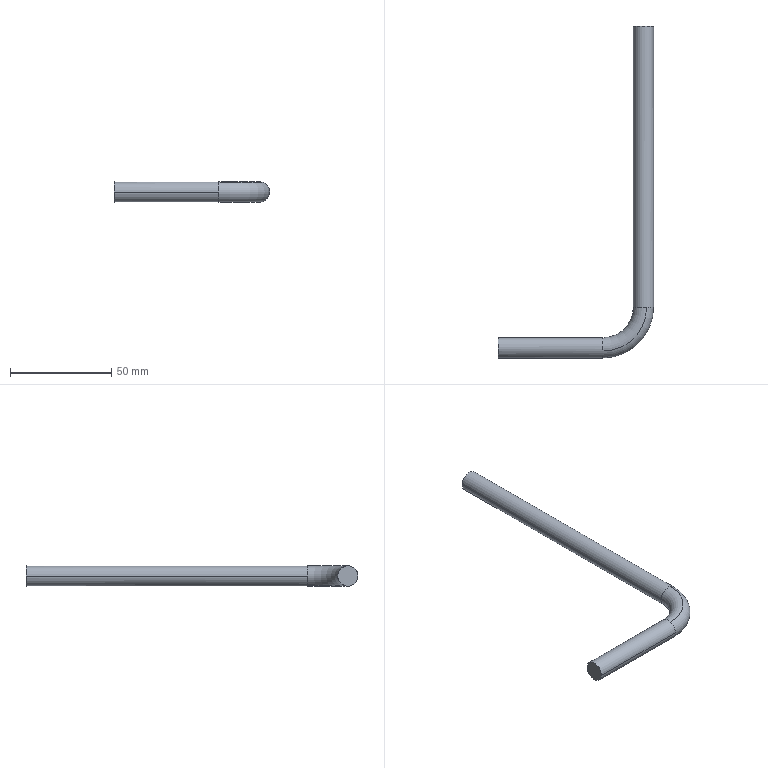Part | 1 solid | 8 faces | box 76.634 x 163.975 x 10 mm | volume 17438 mm3 | cylinder 4 | plane 2 | torus 2 | commonest cylinder face diameters 10 x4
STEP:
#1=CARTESIAN_POINT('',(0.,0.,0.));
#2=DIRECTION('',(0.,0.,1.));
#3=DIRECTION('',(1.,0.,0.));
#4=AXIS2_PLACEMENT_3D('',#1,#2,#3);
#5=CARTESIAN_POINT('',(-430.236,381.551,-68.051));
#6=VERTEX_POINT('',#5);
#7=CARTESIAN_POINT('',(-430.236,520.526,-68.051));
#8=VERTEX_POINT('',#7);
#9=CARTESIAN_POINT('',(-430.236,381.551,-68.051));
#10=DIRECTION('',(0.,1.,0.));
#11=VECTOR('',#10,1.);
#12=LINE('',#9,#11);
#13=CARTESIAN_POINT('',(-425.236,381.551,-68.051));
#14=DIRECTION('',(0.,1.,0.));
#15=DIRECTION('',(0.,0.,-1.));
#16=AXIS2_PLACEMENT_3D('',#13,#14,#15);
#17=CYLINDRICAL_SURFACE('',#16,5.);
#18=CARTESIAN_POINT('',(1.571,0.));
#19=DIRECTION('',(0.,1.));
#20=VECTOR('',#19,1.);
#21=LINE('',#18,#20);
#22=(GEOMETRIC_REPRESENTATION_CONTEXT(2)PARAMETRIC_REPRESENTATION_CONTEXT()REPRESENTATION_CONTEXT('',''));
#23=DEFINITIONAL_REPRESENTATION('',(#21),#22);
#24=PCURVE('',#17,#23);
#25=CARTESIAN_POINT('',(-425.236,381.551,-68.051));
#26=DIRECTION('',(0.,1.,0.));
#27=DIRECTION('',(0.,0.,1.));
#28=AXIS2_PLACEMENT_3D('',#25,#26,#27);
#29=CYLINDRICAL_SURFACE('',#28,5.);
#30=CARTESIAN_POINT('',(4.712,0.));
#31=DIRECTION('',(0.,1.));
#32=VECTOR('',#31,1.);
#33=LINE('',#30,#32);
#34=(GEOMETRIC_REPRESENTATION_CONTEXT(2)PARAMETRIC_REPRESENTATION_CONTEXT()REPRESENTATION_CONTEXT('',''));
#35=DEFINITIONAL_REPRESENTATION('',(#33),#34);
#36=PCURVE('',#29,#35);
#37=SURFACE_CURVE('',#12,(#24,#36),.PCURVE_S1.);
#38=EDGE_CURVE('',#6,#8,#37,.T.);
#39=ORIENTED_EDGE('',*,*,#38,.F.);
#40=CARTESIAN_POINT('',(-423.691,381.551,-63.296));
#41=VERTEX_POINT('',#40);
#42=CARTESIAN_POINT('',(-425.236,381.551,-68.051));
#43=DIRECTION('',(0.,1.,0.));
#44=DIRECTION('',(1.,0.,0.));
#45=AXIS2_PLACEMENT_3D('',#42,#43,#44);
#46=CIRCLE('',#45,5.);
#47=CARTESIAN_POINT('',(-1.571,0.));
#48=DIRECTION('',(1.,0.));
#49=VECTOR('',#48,1.);
#50=LINE('',#47,#49);
#51=(GEOMETRIC_REPRESENTATION_CONTEXT(2)PARAMETRIC_REPRESENTATION_CONTEXT()REPRESENTATION_CONTEXT('',''));
#52=DEFINITIONAL_REPRESENTATION('',(#50),#51);
#53=PCURVE('',#17,#52);
#54=CARTESIAN_POINT('',(-445.236,381.551,-68.051));
#55=DIRECTION('',(0.,0.,1.));
#56=DIRECTION('',(-0.7071,0.7071,0.));
#57=AXIS2_PLACEMENT_3D('',#54,#55,#56);
#58=TOROIDAL_SURFACE('',#57,20.,5.);
#59=CARTESIAN_POINT('',(3.927,6.283));
#60=DIRECTION('',(0.,-1.));
#61=VECTOR('',#60,1.);
#62=LINE('',#59,#61);
#63=(GEOMETRIC_REPRESENTATION_CONTEXT(2)PARAMETRIC_REPRESENTATION_CONTEXT()REPRESENTATION_CONTEXT('',''));
#64=DEFINITIONAL_REPRESENTATION('',(#62),#63);
#65=PCURVE('',#58,#64);
#66=SURFACE_CURVE('',#46,(#53,#65),.PCURVE_S1.);
#67=EDGE_CURVE('',#6,#41,#66,.T.);
#68=ORIENTED_EDGE('',*,*,#67,.T.);
#69=CARTESIAN_POINT('',(-420.236,381.551,-68.051));
#70=VERTEX_POINT('',#69);
#71=CARTESIAN_POINT('',(-425.236,381.551,-68.051));
#72=DIRECTION('',(0.,1.,0.));
#73=DIRECTION('',(1.,0.,0.));
#74=AXIS2_PLACEMENT_3D('',#71,#72,#73);
#75=CIRCLE('',#74,5.);
#76=CARTESIAN_POINT('',(-1.571,0.));
#77=DIRECTION('',(1.,0.));
#78=VECTOR('',#77,1.);
#79=LINE('',#76,#78);
#80=(GEOMETRIC_REPRESENTATION_CONTEXT(2)PARAMETRIC_REPRESENTATION_CONTEXT()REPRESENTATION_CONTEXT('',''));
#81=DEFINITIONAL_REPRESENTATION('',(#79),#80);
#82=PCURVE('',#17,#81);
#83=CARTESIAN_POINT('',(-445.236,381.551,-68.051));
#84=DIRECTION('',(0.,0.,1.));
#85=DIRECTION('',(-0.7071,0.7071,0.));
#86=AXIS2_PLACEMENT_3D('',#83,#84,#85);
#87=TOROIDAL_SURFACE('',#86,20.,5.);
#88=CARTESIAN_POINT('',(3.927,12.566));
#89=DIRECTION('',(0.,-1.));
#90=VECTOR('',#89,1.);
#91=LINE('',#88,#90);
#92=(GEOMETRIC_REPRESENTATION_CONTEXT(2)PARAMETRIC_REPRESENTATION_CONTEXT()REPRESENTATION_CONTEXT('',''));
#93=DEFINITIONAL_REPRESENTATION('',(#91),#92);
#94=PCURVE('',#87,#93);
#95=SURFACE_CURVE('',#75,(#82,#94),.PCURVE_S1.);
#96=EDGE_CURVE('',#41,#70,#95,.T.);
#97=ORIENTED_EDGE('',*,*,#96,.T.);
#98=CARTESIAN_POINT('',(-420.236,520.526,-68.051));
#99=VERTEX_POINT('',#98);
#100=CARTESIAN_POINT('',(-420.236,381.551,-68.051));
#101=DIRECTION('',(0.,1.,0.));
#102=VECTOR('',#101,1.);
#103=LINE('',#100,#102);
#104=CARTESIAN_POINT('',(4.712,0.));
#105=DIRECTION('',(0.,1.));
#106=VECTOR('',#105,1.);
#107=LINE('',#104,#106);
#108=(GEOMETRIC_REPRESENTATION_CONTEXT(2)PARAMETRIC_REPRESENTATION_CONTEXT()REPRESENTATION_CONTEXT('',''));
#109=DEFINITIONAL_REPRESENTATION('',(#107),#108);
#110=PCURVE('',#17,#109);
#111=CARTESIAN_POINT('',(1.571,0.));
#112=DIRECTION('',(0.,1.));
#113=VECTOR('',#112,1.);
#114=LINE('',#111,#113);
#115=(GEOMETRIC_REPRESENTATION_CONTEXT(2)PARAMETRIC_REPRESENTATION_CONTEXT()REPRESENTATION_CONTEXT('',''));
#116=DEFINITIONAL_REPRESENTATION('',(#114),#115);
#117=PCURVE('',#29,#116);
#118=SURFACE_CURVE('',#103,(#110,#117),.PCURVE_S1.);
#119=EDGE_CURVE('',#70,#99,#118,.T.);
#120=ORIENTED_EDGE('',*,*,#119,.T.);
#121=CARTESIAN_POINT('',(-425.236,520.526,-68.051));
#122=DIRECTION('',(0.,1.,0.));
#123=DIRECTION('',(1.,0.,0.));
#124=AXIS2_PLACEMENT_3D('',#121,#122,#123);
#125=CIRCLE('',#124,5.);
#126=CARTESIAN_POINT('',(-1.571,138.975));
#127=DIRECTION('',(1.,0.));
#128=VECTOR('',#127,1.);
#129=LINE('',#126,#128);
#130=(GEOMETRIC_REPRESENTATION_CONTEXT(2)PARAMETRIC_REPRESENTATION_CONTEXT()REPRESENTATION_CONTEXT('',''));
#131=DEFINITIONAL_REPRESENTATION('',(#129),#130);
#132=PCURVE('',#17,#131);
#133=CARTESIAN_POINT('',(-402.025,520.526,-111.002));
#134=DIRECTION('',(0.,-1.,0.));
#135=DIRECTION('',(-1.,0.,0.));
#136=AXIS2_PLACEMENT_3D('',#133,#134,#135);
#137=PLANE('',#136);
#138=CARTESIAN_POINT('',(18.211,-42.951));
#139=CARTESIAN_POINT('',(18.211,-34.291));
#140=CARTESIAN_POINT('',(25.711,-38.621));
#141=CARTESIAN_POINT('',(33.211,-42.951));
#142=CARTESIAN_POINT('',(25.711,-47.281));
#143=CARTESIAN_POINT('',(18.211,-51.611));
#144=CARTESIAN_POINT('',(18.211,-42.951));
#145=(BOUNDED_CURVE()B_SPLINE_CURVE(2,(#138,#139,#140,#141,#142,#143,#144),.UNSPECIFIED.,.T.,.F.)B_SPLINE_CURVE_WITH_KNOTS((1,2,2,2,2,1),(-2.094,0.,2.094,4.189,6.283,8.378),.UNSPECIFIED.)CURVE()GEOMETRIC_REPRESENTATION_ITEM()RATIONAL_B_SPLINE_CURVE((1.,0.5,1.,0.5,1.,0.5,1.))REPRESENTATION_ITEM(''));
#146=(GEOMETRIC_REPRESENTATION_CONTEXT(2)PARAMETRIC_REPRESENTATION_CONTEXT()REPRESENTATION_CONTEXT('',''));
#147=DEFINITIONAL_REPRESENTATION('',(#145),#146);
#148=PCURVE('',#137,#147);
#149=SURFACE_CURVE('',#125,(#132,#148),.PCURVE_S1.);
#150=EDGE_CURVE('',#8,#99,#149,.T.);
#151=ORIENTED_EDGE('',*,*,#150,.F.);
#152=EDGE_LOOP('',(#39,#68,#97,#120,#151));
#153=FACE_BOUND('',#152,.T.);
#154=ADVANCED_FACE('',(#153),#17,.T.);
#155=CARTESIAN_POINT('',(-425.236,520.526,-68.051));
#156=DIRECTION('',(0.,1.,0.));
#157=DIRECTION('',(1.,0.,0.));
#158=AXIS2_PLACEMENT_3D('',#155,#156,#157);
#159=CIRCLE('',#158,5.);
#160=CARTESIAN_POINT('',(18.211,-42.951));
#161=CARTESIAN_POINT('',(18.211,-34.291));
#162=CARTESIAN_POINT('',(25.711,-38.621));
#163=CARTESIAN_POINT('',(33.211,-42.951));
#164=CARTESIAN_POINT('',(25.711,-47.281));
#165=CARTESIAN_POINT('',(18.211,-51.611));
#166=CARTESIAN_POINT('',(18.211,-42.951));
#167=(BOUNDED_CURVE()B_SPLINE_CURVE(2,(#160,#161,#162,#163,#164,#165,#166),.UNSPECIFIED.,.T.,.F.)B_SPLINE_CURVE_WITH_KNOTS((1,2,2,2,2,1),(-2.094,0.,2.094,4.189,6.283,8.378),.UNSPECIFIED.)CURVE()GEOMETRIC_REPRESENTATION_ITEM()RATIONAL_B_SPLINE_CURVE((1.,0.5,1.,0.5,1.,0.5,1.))REPRESENTATION_ITEM(''));
#168=(GEOMETRIC_REPRESENTATION_CONTEXT(2)PARAMETRIC_REPRESENTATION_CONTEXT()REPRESENTATION_CONTEXT('',''));
#169=DEFINITIONAL_REPRESENTATION('',(#167),#168);
#170=PCURVE('',#137,#169);
#171=CARTESIAN_POINT('',(1.571,138.975));
#172=DIRECTION('',(1.,0.));
#173=VECTOR('',#172,1.);
#174=LINE('',#171,#173);
#175=(GEOMETRIC_REPRESENTATION_CONTEXT(2)PARAMETRIC_REPRESENTATION_CONTEXT()REPRESENTATION_CONTEXT('',''));
#176=DEFINITIONAL_REPRESENTATION('',(#174),#175);
#177=PCURVE('',#29,#176);
#178=SURFACE_CURVE('',#159,(#170,#177),.PCURVE_S1.);
#179=EDGE_CURVE('',#99,#8,#178,.T.);
#180=ORIENTED_EDGE('',*,*,#179,.T.);
#181=ORIENTED_EDGE('',*,*,#150,.T.);
#182=EDGE_LOOP('',(#180,#181));
#183=FACE_BOUND('',#182,.T.);
#184=ADVANCED_FACE('',(#183),#137,.F.);
#185=CARTESIAN_POINT('',(-445.236,363.096,-72.807));
#186=VERTEX_POINT('',#185);
#187=CARTESIAN_POINT('',(-426.781,381.551,-72.807));
#188=VERTEX_POINT('',#187);
#189=CARTESIAN_POINT('',(-445.236,381.551,-72.807));
#190=DIRECTION('',(0.,0.,1.));
#191=DIRECTION('',(0.,-1.,0.));
#192=AXIS2_PLACEMENT_3D('',#189,#190,#191);
#193=CIRCLE('',#192,18.455);
#194=CARTESIAN_POINT('',(2.356,4.398));
#195=DIRECTION('',(1.,0.));
#196=VECTOR('',#195,1.);
#197=LINE('',#194,#196);
#198=(GEOMETRIC_REPRESENTATION_CONTEXT(2)PARAMETRIC_REPRESENTATION_CONTEXT()REPRESENTATION_CONTEXT('',''));
#199=DEFINITIONAL_REPRESENTATION('',(#197),#198);
#200=PCURVE('',#58,#199);
#201=CARTESIAN_POINT('',(2.356,4.398));
#202=DIRECTION('',(1.,0.));
#203=VECTOR('',#202,1.);
#204=LINE('',#201,#203);
#205=(GEOMETRIC_REPRESENTATION_CONTEXT(2)PARAMETRIC_REPRESENTATION_CONTEXT()REPRESENTATION_CONTEXT('',''));
#206=DEFINITIONAL_REPRESENTATION('',(#204),#205);
#207=PCURVE('',#87,#206);
#208=SURFACE_CURVE('',#193,(#200,#207),.PCURVE_S1.);
#209=EDGE_CURVE('',#186,#188,#208,.T.);
#210=ORIENTED_EDGE('',*,*,#209,.F.);
#211=CARTESIAN_POINT('',(-445.236,366.551,-68.051));
#212=VERTEX_POINT('',#211);
#213=CARTESIAN_POINT('',(-445.236,361.551,-68.051));
#214=DIRECTION('',(1.,0.,0.));
#215=DIRECTION('',(0.,1.,0.));
#216=AXIS2_PLACEMENT_3D('',#213,#214,#215);
#217=CIRCLE('',#216,5.);
#218=CARTESIAN_POINT('',(2.356,9.425));
#219=DIRECTION('',(0.,-1.));
#220=VECTOR('',#219,1.);
#221=LINE('',#218,#220);
#222=(GEOMETRIC_REPRESENTATION_CONTEXT(2)PARAMETRIC_REPRESENTATION_CONTEXT()REPRESENTATION_CONTEXT('',''));
#223=DEFINITIONAL_REPRESENTATION('',(#221),#222);
#224=PCURVE('',#58,#223);
#225=CARTESIAN_POINT('',(-445.236,361.551,-68.051));
#226=DIRECTION('',(-1.,0.,0.));
#227=DIRECTION('',(0.,0.,1.));
#228=AXIS2_PLACEMENT_3D('',#225,#226,#227);
#229=CYLINDRICAL_SURFACE('',#228,5.);
#230=CARTESIAN_POINT('',(7.854,0.));
#231=DIRECTION('',(-1.,0.));
#232=VECTOR('',#231,1.);
#233=LINE('',#230,#232);
#234=(GEOMETRIC_REPRESENTATION_CONTEXT(2)PARAMETRIC_REPRESENTATION_CONTEXT()REPRESENTATION_CONTEXT('',''));
#235=DEFINITIONAL_REPRESENTATION('',(#233),#234);
#236=PCURVE('',#229,#235);
#237=SURFACE_CURVE('',#217,(#224,#236),.PCURVE_S1.);
#238=EDGE_CURVE('',#186,#212,#237,.T.);
#239=ORIENTED_EDGE('',*,*,#238,.T.);
#240=CARTESIAN_POINT('',(-445.236,360.006,-63.296));
#241=VERTEX_POINT('',#240);
#242=CARTESIAN_POINT('',(-445.236,361.551,-68.051));
#243=DIRECTION('',(1.,0.,0.));
#244=DIRECTION('',(0.,1.,0.));
#245=AXIS2_PLACEMENT_3D('',#242,#243,#244);
#246=CIRCLE('',#245,5.);
#247=CARTESIAN_POINT('',(2.356,3.142));
#248=DIRECTION('',(0.,-1.));
#249=VECTOR('',#248,1.);
#250=LINE('',#247,#249);
#251=(GEOMETRIC_REPRESENTATION_CONTEXT(2)PARAMETRIC_REPRESENTATION_CONTEXT()REPRESENTATION_CONTEXT('',''));
#252=DEFINITIONAL_REPRESENTATION('',(#250),#251);
#253=PCURVE('',#58,#252);
#254=CARTESIAN_POINT('',(-445.236,361.551,-68.051));
#255=DIRECTION('',(-1.,0.,0.));
#256=DIRECTION('',(0.,0.,-1.));
#257=AXIS2_PLACEMENT_3D('',#254,#255,#256);
#258=CYLINDRICAL_SURFACE('',#257,5.);
#259=CARTESIAN_POINT('',(4.712,0.));
#260=DIRECTION('',(-1.,0.));
#261=VECTOR('',#260,1.);
#262=LINE('',#259,#261);
#263=(GEOMETRIC_REPRESENTATION_CONTEXT(2)PARAMETRIC_REPRESENTATION_CONTEXT()REPRESENTATION_CONTEXT('',''));
#264=DEFINITIONAL_REPRESENTATION('',(#262),#263);
#265=PCURVE('',#258,#264);
#266=SURFACE_CURVE('',#246,(#253,#265),.PCURVE_S1.);
#267=EDGE_CURVE('',#212,#241,#266,.T.);
#268=ORIENTED_EDGE('',*,*,#267,.T.);
#269=CARTESIAN_POINT('',(-445.236,381.551,-63.296));
#270=DIRECTION('',(0.,0.,1.));
#271=DIRECTION('',(0.,-1.,0.));
#272=AXIS2_PLACEMENT_3D('',#269,#270,#271);
#273=CIRCLE('',#272,21.545);
#274=CARTESIAN_POINT('',(2.356,1.257));
#275=DIRECTION('',(1.,0.));
#276=VECTOR('',#275,1.);
#277=LINE('',#274,#276);
#278=(GEOMETRIC_REPRESENTATION_CONTEXT(2)PARAMETRIC_REPRESENTATION_CONTEXT()REPRESENTATION_CONTEXT('',''));
#279=DEFINITIONAL_REPRESENTATION('',(#277),#278);
#280=PCURVE('',#58,#279);
#281=CARTESIAN_POINT('',(2.356,7.54));
#282=DIRECTION('',(1.,0.));
#283=VECTOR('',#282,1.);
#284=LINE('',#281,#283);
#285=(GEOMETRIC_REPRESENTATION_CONTEXT(2)PARAMETRIC_REPRESENTATION_CONTEXT()REPRESENTATION_CONTEXT('',''));
#286=DEFINITIONAL_REPRESENTATION('',(#284),#285);
#287=PCURVE('',#87,#286);
#288=SURFACE_CURVE('',#273,(#280,#287),.PCURVE_S1.);
#289=EDGE_CURVE('',#241,#41,#288,.T.);
#290=ORIENTED_EDGE('',*,*,#289,.T.);
#291=ORIENTED_EDGE('',*,*,#67,.F.);
#292=CARTESIAN_POINT('',(-425.236,381.551,-68.051));
#293=DIRECTION('',(0.,1.,0.));
#294=DIRECTION('',(1.,0.,0.));
#295=AXIS2_PLACEMENT_3D('',#292,#293,#294);
#296=CIRCLE('',#295,5.);
#297=CARTESIAN_POINT('',(3.927,6.283));
#298=DIRECTION('',(0.,-1.));
#299=VECTOR('',#298,1.);
#300=LINE('',#297,#299);
#301=(GEOMETRIC_REPRESENTATION_CONTEXT(2)PARAMETRIC_REPRESENTATION_CONTEXT()REPRESENTATION_CONTEXT('',''));
#302=DEFINITIONAL_REPRESENTATION('',(#300),#301);
#303=PCURVE('',#58,#302);
#304=CARTESIAN_POINT('',(1.571,0.));
#305=DIRECTION('',(1.,0.));
#306=VECTOR('',#305,1.);
#307=LINE('',#304,#306);
#308=(GEOMETRIC_REPRESENTATION_CONTEXT(2)PARAMETRIC_REPRESENTATION_CONTEXT()REPRESENTATION_CONTEXT('',''));
#309=DEFINITIONAL_REPRESENTATION('',(#307),#308);
#310=PCURVE('',#29,#309);
#311=SURFACE_CURVE('',#296,(#303,#310),.PCURVE_S1.);
#312=EDGE_CURVE('',#188,#6,#311,.T.);
#313=ORIENTED_EDGE('',*,*,#312,.F.);
#314=EDGE_LOOP('',(#210,#239,#268,#290,#291,#313));
#315=FACE_BOUND('',#314,.T.);
#316=ADVANCED_FACE('',(#315),#58,.T.);
#317=CARTESIAN_POINT('',(-445.236,356.551,-68.051));
#318=VERTEX_POINT('',#317);
#319=CARTESIAN_POINT('',(-496.87,356.551,-68.051));
#320=VERTEX_POINT('',#319);
#321=CARTESIAN_POINT('',(-445.236,356.551,-68.051));
#322=DIRECTION('',(-1.,0.,0.));
#323=VECTOR('',#322,1.);
#324=LINE('',#321,#323);
#325=CARTESIAN_POINT('',(1.571,0.));
#326=DIRECTION('',(0.,1.));
#327=VECTOR('',#326,1.);
#328=LINE('',#325,#327);
#329=(GEOMETRIC_REPRESENTATION_CONTEXT(2)PARAMETRIC_REPRESENTATION_CONTEXT()REPRESENTATION_CONTEXT('',''));
#330=DEFINITIONAL_REPRESENTATION('',(#328),#329);
#331=PCURVE('',#258,#330);
#332=CARTESIAN_POINT('',(4.712,0.));
#333=DIRECTION('',(0.,1.));
#334=VECTOR('',#333,1.);
#335=LINE('',#332,#334);
#336=(GEOMETRIC_REPRESENTATION_CONTEXT(2)PARAMETRIC_REPRESENTATION_CONTEXT()REPRESENTATION_CONTEXT('',''));
#337=DEFINITIONAL_REPRESENTATION('',(#335),#336);
#338=PCURVE('',#229,#337);
#339=SURFACE_CURVE('',#324,(#331,#338),.PCURVE_S1.);
#340=EDGE_CURVE('',#318,#320,#339,.T.);
#341=ORIENTED_EDGE('',*,*,#340,.F.);
#342=CARTESIAN_POINT('',(-445.236,361.551,-68.051));
#343=DIRECTION('',(1.,0.,0.));
#344=DIRECTION('',(0.,1.,0.));
#345=AXIS2_PLACEMENT_3D('',#342,#343,#344);
#346=CIRCLE('',#345,5.);
#347=CARTESIAN_POINT('',(4.712,0.));
#348=DIRECTION('',(-1.,0.));
#349=VECTOR('',#348,1.);
#350=LINE('',#347,#349);
#351=(GEOMETRIC_REPRESENTATION_CONTEXT(2)PARAMETRIC_REPRESENTATION_CONTEXT()REPRESENTATION_CONTEXT('',''));
#352=DEFINITIONAL_REPRESENTATION('',(#350),#351);
#353=PCURVE('',#258,#352);
#354=CARTESIAN_POINT('',(2.356,9.425));
#355=DIRECTION('',(0.,-1.));
#356=VECTOR('',#355,1.);
#357=LINE('',#354,#356);
#358=(GEOMETRIC_REPRESENTATION_CONTEXT(2)PARAMETRIC_REPRESENTATION_CONTEXT()REPRESENTATION_CONTEXT('',''));
#359=DEFINITIONAL_REPRESENTATION('',(#357),#358);
#360=PCURVE('',#87,#359);
#361=SURFACE_CURVE('',#346,(#353,#360),.PCURVE_S1.);
#362=EDGE_CURVE('',#241,#318,#361,.T.);
#363=ORIENTED_EDGE('',*,*,#362,.F.);
#364=ORIENTED_EDGE('',*,*,#267,.F.);
#365=CARTESIAN_POINT('',(-496.87,366.551,-68.051));
#366=VERTEX_POINT('',#365);
#367=CARTESIAN_POINT('',(-445.236,366.551,-68.051));
#368=DIRECTION('',(-1.,0.,0.));
#369=VECTOR('',#368,1.);
#370=LINE('',#367,#369);
#371=CARTESIAN_POINT('',(4.712,0.));
#372=DIRECTION('',(0.,1.));
#373=VECTOR('',#372,1.);
#374=LINE('',#371,#373);
#375=(GEOMETRIC_REPRESENTATION_CONTEXT(2)PARAMETRIC_REPRESENTATION_CONTEXT()REPRESENTATION_CONTEXT('',''));
#376=DEFINITIONAL_REPRESENTATION('',(#374),#375);
#377=PCURVE('',#258,#376);
#378=CARTESIAN_POINT('',(1.571,0.));
#379=DIRECTION('',(0.,1.));
#380=VECTOR('',#379,1.);
#381=LINE('',#378,#380);
#382=(GEOMETRIC_REPRESENTATION_CONTEXT(2)PARAMETRIC_REPRESENTATION_CONTEXT()REPRESENTATION_CONTEXT('',''));
#383=DEFINITIONAL_REPRESENTATION('',(#381),#382);
#384=PCURVE('',#229,#383);
#385=SURFACE_CURVE('',#370,(#377,#384),.PCURVE_S1.);
#386=EDGE_CURVE('',#212,#366,#385,.T.);
#387=ORIENTED_EDGE('',*,*,#386,.T.);
#388=CARTESIAN_POINT('',(-496.87,361.551,-68.051));
#389=DIRECTION('',(1.,0.,0.));
#390=DIRECTION('',(0.,1.,0.));
#391=AXIS2_PLACEMENT_3D('',#388,#389,#390);
#392=CIRCLE('',#391,5.);
#393=CARTESIAN_POINT('',(4.712,51.634));
#394=DIRECTION('',(-1.,0.));
#395=VECTOR('',#394,1.);
#396=LINE('',#393,#395);
#397=(GEOMETRIC_REPRESENTATION_CONTEXT(2)PARAMETRIC_REPRESENTATION_CONTEXT()REPRESENTATION_CONTEXT('',''));
#398=DEFINITIONAL_REPRESENTATION('',(#396),#397);
#399=PCURVE('',#258,#398);
#400=CARTESIAN_POINT('',(-496.87,361.551,-68.051));
#401=DIRECTION('',(1.,0.,0.));
#402=DIRECTION('',(0.,-1.,0.));
#403=AXIS2_PLACEMENT_3D('',#400,#401,#402);
#404=PLANE('',#403);
#405=CARTESIAN_POINT('',(0.,0.));
#406=DIRECTION('',(-1.,0.));
#407=AXIS2_PLACEMENT_2D('',#405,#406);
#408=CIRCLE('',#407,5.);
#409=(GEOMETRIC_REPRESENTATION_CONTEXT(2)PARAMETRIC_REPRESENTATION_CONTEXT()REPRESENTATION_CONTEXT('',''));
#410=DEFINITIONAL_REPRESENTATION('',(#408),#409);
#411=PCURVE('',#404,#410);
#412=SURFACE_CURVE('',#392,(#399,#411),.PCURVE_S1.);
#413=EDGE_CURVE('',#366,#320,#412,.T.);
#414=ORIENTED_EDGE('',*,*,#413,.T.);
#415=EDGE_LOOP('',(#341,#363,#364,#387,#414));
#416=FACE_BOUND('',#415,.T.);
#417=ADVANCED_FACE('',(#416),#258,.T.);
#418=CARTESIAN_POINT('',(-496.87,361.551,-68.051));
#419=DIRECTION('',(1.,0.,0.));
#420=DIRECTION('',(0.,1.,0.));
#421=AXIS2_PLACEMENT_3D('',#418,#419,#420);
#422=CIRCLE('',#421,5.);
#423=CARTESIAN_POINT('',(0.,0.));
#424=DIRECTION('',(-1.,0.));
#425=AXIS2_PLACEMENT_2D('',#423,#424);
#426=CIRCLE('',#425,5.);
#427=(GEOMETRIC_REPRESENTATION_CONTEXT(2)PARAMETRIC_REPRESENTATION_CONTEXT()REPRESENTATION_CONTEXT('',''));
#428=DEFINITIONAL_REPRESENTATION('',(#426),#427);
#429=PCURVE('',#404,#428);
#430=CARTESIAN_POINT('',(7.854,51.634));
#431=DIRECTION('',(-1.,0.));
#432=VECTOR('',#431,1.);
#433=LINE('',#430,#432);
#434=(GEOMETRIC_REPRESENTATION_CONTEXT(2)PARAMETRIC_REPRESENTATION_CONTEXT()REPRESENTATION_CONTEXT('',''));
#435=DEFINITIONAL_REPRESENTATION('',(#433),#434);
#436=PCURVE('',#229,#435);
#437=SURFACE_CURVE('',#422,(#429,#436),.PCURVE_S1.);
#438=EDGE_CURVE('',#320,#366,#437,.T.);
#439=ORIENTED_EDGE('',*,*,#438,.F.);
#440=ORIENTED_EDGE('',*,*,#413,.F.);
#441=EDGE_LOOP('',(#439,#440));
#442=FACE_BOUND('',#441,.T.);
#443=ADVANCED_FACE('',(#442),#404,.F.);
#444=ORIENTED_EDGE('',*,*,#38,.T.);
#445=ORIENTED_EDGE('',*,*,#179,.F.);
#446=ORIENTED_EDGE('',*,*,#119,.F.);
#447=CARTESIAN_POINT('',(-425.236,381.551,-68.051));
#448=DIRECTION('',(0.,1.,0.));
#449=DIRECTION('',(1.,0.,0.));
#450=AXIS2_PLACEMENT_3D('',#447,#448,#449);
#451=CIRCLE('',#450,5.);
#452=CARTESIAN_POINT('',(1.571,0.));
#453=DIRECTION('',(1.,0.));
#454=VECTOR('',#453,1.);
#455=LINE('',#452,#454);
#456=(GEOMETRIC_REPRESENTATION_CONTEXT(2)PARAMETRIC_REPRESENTATION_CONTEXT()REPRESENTATION_CONTEXT('',''));
#457=DEFINITIONAL_REPRESENTATION('',(#455),#456);
#458=PCURVE('',#29,#457);
#459=CARTESIAN_POINT('',(3.927,6.283));
#460=DIRECTION('',(0.,-1.));
#461=VECTOR('',#460,1.);
#462=LINE('',#459,#461);
#463=(GEOMETRIC_REPRESENTATION_CONTEXT(2)PARAMETRIC_REPRESENTATION_CONTEXT()REPRESENTATION_CONTEXT('',''));
#464=DEFINITIONAL_REPRESENTATION('',(#462),#463);
#465=PCURVE('',#87,#464);
#466=SURFACE_CURVE('',#451,(#458,#465),.PCURVE_S1.);
#467=EDGE_CURVE('',#70,#188,#466,.T.);
#468=ORIENTED_EDGE('',*,*,#467,.T.);
#469=ORIENTED_EDGE('',*,*,#312,.T.);
#470=EDGE_LOOP('',(#444,#445,#446,#468,#469));
#471=FACE_BOUND('',#470,.T.);
#472=ADVANCED_FACE('',(#471),#29,.T.);
#473=ORIENTED_EDGE('',*,*,#209,.T.);
#474=ORIENTED_EDGE('',*,*,#467,.F.);
#475=ORIENTED_EDGE('',*,*,#96,.F.);
#476=ORIENTED_EDGE('',*,*,#289,.F.);
#477=ORIENTED_EDGE('',*,*,#362,.T.);
#478=CARTESIAN_POINT('',(-445.236,361.551,-68.051));
#479=DIRECTION('',(1.,0.,0.));
#480=DIRECTION('',(0.,1.,0.));
#481=AXIS2_PLACEMENT_3D('',#478,#479,#480);
#482=CIRCLE('',#481,5.);
#483=CARTESIAN_POINT('',(2.356,9.425));
#484=DIRECTION('',(0.,-1.));
#485=VECTOR('',#484,1.);
#486=LINE('',#483,#485);
#487=(GEOMETRIC_REPRESENTATION_CONTEXT(2)PARAMETRIC_REPRESENTATION_CONTEXT()REPRESENTATION_CONTEXT('',''));
#488=DEFINITIONAL_REPRESENTATION('',(#486),#487);
#489=PCURVE('',#87,#488);
#490=CARTESIAN_POINT('',(7.854,0.));
#491=DIRECTION('',(-1.,0.));
#492=VECTOR('',#491,1.);
#493=LINE('',#490,#492);
#494=(GEOMETRIC_REPRESENTATION_CONTEXT(2)PARAMETRIC_REPRESENTATION_CONTEXT()REPRESENTATION_CONTEXT('',''));
#495=DEFINITIONAL_REPRESENTATION('',(#493),#494);
#496=PCURVE('',#229,#495);
#497=SURFACE_CURVE('',#482,(#489,#496),.PCURVE_S1.);
#498=EDGE_CURVE('',#318,#186,#497,.T.);
#499=ORIENTED_EDGE('',*,*,#498,.T.);
#500=EDGE_LOOP('',(#473,#474,#475,#476,#477,#499));
#501=FACE_BOUND('',#500,.T.);
#502=ADVANCED_FACE('',(#501),#87,.T.);
#503=ORIENTED_EDGE('',*,*,#340,.T.);
#504=ORIENTED_EDGE('',*,*,#438,.T.);
#505=ORIENTED_EDGE('',*,*,#386,.F.);
#506=ORIENTED_EDGE('',*,*,#238,.F.);
#507=ORIENTED_EDGE('',*,*,#498,.F.);
#508=EDGE_LOOP('',(#503,#504,#505,#506,#507));
#509=FACE_BOUND('',#508,.T.);
#510=ADVANCED_FACE('',(#509),#229,.T.);
#511=CLOSED_SHELL('',(#154,#184,#316,#417,#443,#472,#502,#510));
#512=MANIFOLD_SOLID_BREP('',#511);
#513=(LENGTH_UNIT()NAMED_UNIT(*)SI_UNIT(.MILLI.,.METRE.));
#514=UNCERTAINTY_MEASURE_WITH_UNIT(LENGTH_MEASURE(0.0000001),#513,'','');
#515=(NAMED_UNIT(*)PLANE_ANGLE_UNIT()SI_UNIT($,.RADIAN.));
#516=(NAMED_UNIT(*)SI_UNIT($,.STERADIAN.)SOLID_ANGLE_UNIT());
#517=(GEOMETRIC_REPRESENTATION_CONTEXT(3)GLOBAL_UNCERTAINTY_ASSIGNED_CONTEXT((#514))GLOBAL_UNIT_ASSIGNED_CONTEXT((#513,#515,#516))REPRESENTATION_CONTEXT('',''));
#518=ADVANCED_BREP_SHAPE_REPRESENTATION('',(#4,#512),#517);